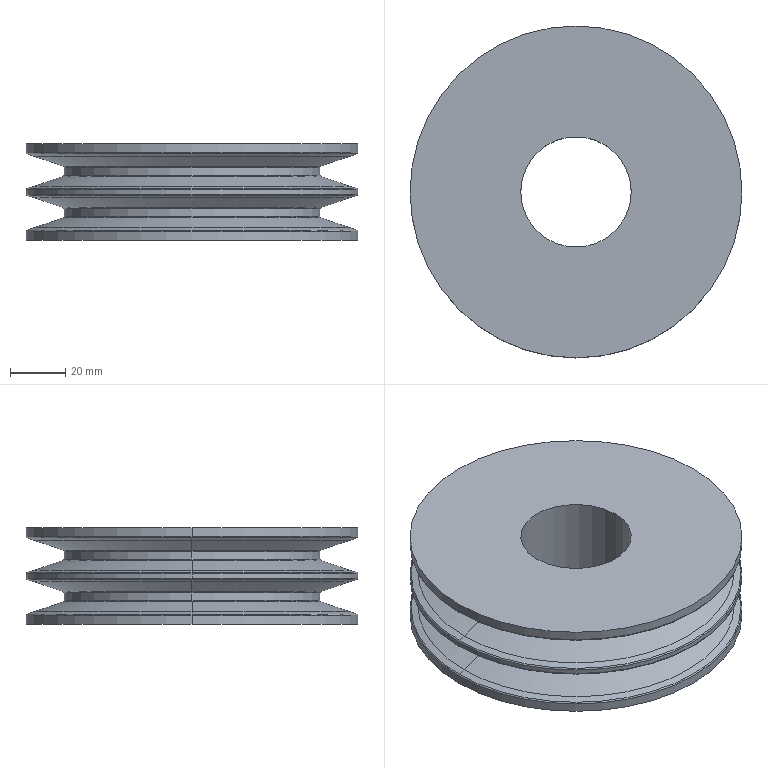Part | SolidWorks | features Extrusion 1, Fillet 1, LPattern 1, RevCut 1 | 1 solid | 46 faces | box 120 x 120 x 35 mm | volume 274896 mm3 | torus 16 | cone 16 | cylinder 12 | plane 2 | commonest cylinder face diameters 120 x6 92.4 x4 40 x2
STEP:
#1=CARTESIAN_POINT('',(-46.537,0.,-5.671));
#2=VERTEX_POINT('',#1);
#3=CARTESIAN_POINT('',(46.537,0.,-5.671));
#4=VERTEX_POINT('',#3);
#5=CARTESIAN_POINT('',(0.,0.,-5.671));
#6=DIRECTION('',(0.,0.,1.));
#7=DIRECTION('',(1.,0.,0.));
#8=AXIS2_PLACEMENT_3D('',#5,#6,#7);
#9=CIRCLE('',#8,46.537);
#10=EDGE_CURVE('',#2,#4,#9,.T.);
#11=ORIENTED_EDGE('',*,*,#10,.F.);
#12=CARTESIAN_POINT('',(-46.2,0.,-6.144));
#13=VERTEX_POINT('',#12);
#14=CARTESIAN_POINT('',(-46.7,0.,-6.144));
#15=DIRECTION('',(0.,1.,0.));
#16=DIRECTION('',(-1.,0.,0.));
#17=AXIS2_PLACEMENT_3D('',#14,#15,#16);
#18=CIRCLE('',#17,0.5);
#19=EDGE_CURVE('',#2,#13,#18,.T.);
#20=ORIENTED_EDGE('',*,*,#19,.T.);
#21=CARTESIAN_POINT('',(46.2,0.,-6.144));
#22=VERTEX_POINT('',#21);
#23=CARTESIAN_POINT('',(0.,0.,-6.144));
#24=DIRECTION('',(0.,0.,-1.));
#25=DIRECTION('',(1.,0.,0.));
#26=AXIS2_PLACEMENT_3D('',#23,#24,#25);
#27=CIRCLE('',#26,46.2);
#28=EDGE_CURVE('',#22,#13,#27,.T.);
#29=ORIENTED_EDGE('',*,*,#28,.F.);
#30=CARTESIAN_POINT('',(46.7,0.,-6.144));
#31=DIRECTION('',(0.,-1.,0.));
#32=DIRECTION('',(0.,0.,-1.));
#33=AXIS2_PLACEMENT_3D('',#30,#31,#32);
#34=CIRCLE('',#33,0.5);
#35=EDGE_CURVE('',#4,#22,#34,.T.);
#36=ORIENTED_EDGE('',*,*,#35,.F.);
#37=EDGE_LOOP('',(#11,#20,#29,#36));
#38=FACE_OUTER_BOUND('',#37,.T.);
#39=CARTESIAN_POINT('',(0.,0.,-6.144));
#40=DIRECTION('',(0.,0.,1.));
#41=DIRECTION('',(1.,0.,0.));
#42=AXIS2_PLACEMENT_3D('',#39,#40,#41);
#43=TOROIDAL_SURFACE('',#42,46.7,0.5);
#44=ADVANCED_FACE('',(#38),#43,.F.);
#45=CARTESIAN_POINT('',(-46.2,0.,-8.856));
#46=VERTEX_POINT('',#45);
#47=CARTESIAN_POINT('',(46.2,0.,-8.856));
#48=VERTEX_POINT('',#47);
#49=CARTESIAN_POINT('',(0.,0.,-8.856));
#50=DIRECTION('',(0.,0.,1.));
#51=DIRECTION('',(1.,0.,0.));
#52=AXIS2_PLACEMENT_3D('',#49,#50,#51);
#53=CIRCLE('',#52,46.2);
#54=EDGE_CURVE('',#46,#48,#53,.T.);
#55=ORIENTED_EDGE('',*,*,#54,.F.);
#56=CARTESIAN_POINT('',(-46.537,0.,-9.329));
#57=VERTEX_POINT('',#56);
#58=CARTESIAN_POINT('',(-46.7,0.,-8.856));
#59=DIRECTION('',(0.,1.,0.));
#60=DIRECTION('',(-1.,0.,0.));
#61=AXIS2_PLACEMENT_3D('',#58,#59,#60);
#62=CIRCLE('',#61,0.5);
#63=EDGE_CURVE('',#46,#57,#62,.T.);
#64=ORIENTED_EDGE('',*,*,#63,.T.);
#65=CARTESIAN_POINT('',(46.537,0.,-9.329));
#66=VERTEX_POINT('',#65);
#67=CARTESIAN_POINT('',(0.,0.,-9.329));
#68=DIRECTION('',(0.,0.,-1.));
#69=DIRECTION('',(-1.,0.,0.));
#70=AXIS2_PLACEMENT_3D('',#67,#68,#69);
#71=CIRCLE('',#70,46.537);
#72=EDGE_CURVE('',#66,#57,#71,.T.);
#73=ORIENTED_EDGE('',*,*,#72,.F.);
#74=CARTESIAN_POINT('',(46.7,0.,-8.856));
#75=DIRECTION('',(0.,-1.,0.));
#76=DIRECTION('',(0.,0.,-1.));
#77=AXIS2_PLACEMENT_3D('',#74,#75,#76);
#78=CIRCLE('',#77,0.5);
#79=EDGE_CURVE('',#48,#66,#78,.T.);
#80=ORIENTED_EDGE('',*,*,#79,.F.);
#81=EDGE_LOOP('',(#55,#64,#73,#80));
#82=FACE_OUTER_BOUND('',#81,.T.);
#83=CARTESIAN_POINT('',(0.,0.,-8.856));
#84=DIRECTION('',(0.,0.,1.));
#85=DIRECTION('',(1.,0.,0.));
#86=AXIS2_PLACEMENT_3D('',#83,#84,#85);
#87=TOROIDAL_SURFACE('',#86,46.7,0.5);
#88=ADVANCED_FACE('',(#82),#87,.F.);
#89=CARTESIAN_POINT('',(60.,0.,-0.7793));
#90=VERTEX_POINT('',#89);
#91=CARTESIAN_POINT('',(-60.,0.,-0.7793));
#92=VERTEX_POINT('',#91);
#93=CARTESIAN_POINT('',(0.,0.,-0.7793));
#94=DIRECTION('',(0.,0.,1.));
#95=DIRECTION('',(-1.,0.,0.));
#96=AXIS2_PLACEMENT_3D('',#93,#94,#95);
#97=CIRCLE('',#96,60.);
#98=EDGE_CURVE('',#90,#92,#97,.T.);
#99=ORIENTED_EDGE('',*,*,#98,.F.);
#100=CARTESIAN_POINT('',(59.645,0.,-1.258));
#101=VERTEX_POINT('',#100);
#102=CARTESIAN_POINT('',(59.5,0.,-0.7793));
#103=DIRECTION('',(0.,1.,0.));
#104=DIRECTION('',(-1.,0.,0.));
#105=AXIS2_PLACEMENT_3D('',#102,#103,#104);
#106=CIRCLE('',#105,0.5);
#107=EDGE_CURVE('',#90,#101,#106,.T.);
#108=ORIENTED_EDGE('',*,*,#107,.T.);
#109=CARTESIAN_POINT('',(-59.645,0.,-1.258));
#110=VERTEX_POINT('',#109);
#111=CARTESIAN_POINT('',(0.,0.,-1.258));
#112=DIRECTION('',(0.,0.,-1.));
#113=DIRECTION('',(1.,0.,0.));
#114=AXIS2_PLACEMENT_3D('',#111,#112,#113);
#115=CIRCLE('',#114,59.645);
#116=EDGE_CURVE('',#110,#101,#115,.T.);
#117=ORIENTED_EDGE('',*,*,#116,.F.);
#118=CARTESIAN_POINT('',(-59.5,0.,-0.7793));
#119=DIRECTION('',(0.,-1.,0.));
#120=DIRECTION('',(0.,0.,-1.));
#121=AXIS2_PLACEMENT_3D('',#118,#119,#120);
#122=CIRCLE('',#121,0.5);
#123=EDGE_CURVE('',#92,#110,#122,.T.);
#124=ORIENTED_EDGE('',*,*,#123,.F.);
#125=EDGE_LOOP('',(#99,#108,#117,#124));
#126=FACE_OUTER_BOUND('',#125,.T.);
#127=CARTESIAN_POINT('',(0.,0.,-0.7793));
#128=DIRECTION('',(0.,0.,-1.));
#129=DIRECTION('',(-1.,0.,0.));
#130=AXIS2_PLACEMENT_3D('',#127,#128,#129);
#131=TOROIDAL_SURFACE('',#130,59.5,0.5);
#132=ADVANCED_FACE('',(#126),#131,.T.);
#133=CARTESIAN_POINT('',(59.645,0.,-13.742));
#134=VERTEX_POINT('',#133);
#135=CARTESIAN_POINT('',(-59.645,0.,-13.742));
#136=VERTEX_POINT('',#135);
#137=CARTESIAN_POINT('',(0.,0.,-13.742));
#138=DIRECTION('',(0.,0.,1.));
#139=DIRECTION('',(-1.,0.,0.));
#140=AXIS2_PLACEMENT_3D('',#137,#138,#139);
#141=CIRCLE('',#140,59.645);
#142=EDGE_CURVE('',#134,#136,#141,.T.);
#143=ORIENTED_EDGE('',*,*,#142,.F.);
#144=CARTESIAN_POINT('',(60.,0.,-14.221));
#145=VERTEX_POINT('',#144);
#146=CARTESIAN_POINT('',(59.5,0.,-14.221));
#147=DIRECTION('',(0.,1.,0.));
#148=DIRECTION('',(-1.,0.,0.));
#149=AXIS2_PLACEMENT_3D('',#146,#147,#148);
#150=CIRCLE('',#149,0.5);
#151=EDGE_CURVE('',#134,#145,#150,.T.);
#152=ORIENTED_EDGE('',*,*,#151,.T.);
#153=CARTESIAN_POINT('',(-60.,0.,-14.221));
#154=VERTEX_POINT('',#153);
#155=CARTESIAN_POINT('',(0.,0.,-14.221));
#156=DIRECTION('',(0.,0.,-1.));
#157=DIRECTION('',(-1.,0.,0.));
#158=AXIS2_PLACEMENT_3D('',#155,#156,#157);
#159=CIRCLE('',#158,60.);
#160=EDGE_CURVE('',#154,#145,#159,.T.);
#161=ORIENTED_EDGE('',*,*,#160,.F.);
#162=CARTESIAN_POINT('',(-59.5,0.,-14.221));
#163=DIRECTION('',(0.,-1.,0.));
#164=DIRECTION('',(0.,0.,-1.));
#165=AXIS2_PLACEMENT_3D('',#162,#163,#164);
#166=CIRCLE('',#165,0.5);
#167=EDGE_CURVE('',#136,#154,#166,.T.);
#168=ORIENTED_EDGE('',*,*,#167,.F.);
#169=EDGE_LOOP('',(#143,#152,#161,#168));
#170=FACE_OUTER_BOUND('',#169,.T.);
#171=CARTESIAN_POINT('',(0.,0.,-14.221));
#172=DIRECTION('',(0.,0.,-1.));
#173=DIRECTION('',(-1.,0.,0.));
#174=AXIS2_PLACEMENT_3D('',#171,#172,#173);
#175=TOROIDAL_SURFACE('',#174,59.5,0.5);
#176=ADVANCED_FACE('',(#170),#175,.T.);
#177=CARTESIAN_POINT('',(57.2,0.,-13.));
#178=VERTEX_POINT('',#177);
#179=CARTESIAN_POINT('',(-57.2,0.,-13.));
#180=VERTEX_POINT('',#179);
#181=CARTESIAN_POINT('',(0.,0.,-13.));
#182=DIRECTION('',(0.,0.,1.));
#183=DIRECTION('',(1.,0.,0.));
#184=AXIS2_PLACEMENT_3D('',#181,#182,#183);
#185=CIRCLE('',#184,57.2);
#186=EDGE_CURVE('',#178,#180,#185,.T.);
#187=ORIENTED_EDGE('',*,*,#186,.F.);
#188=CARTESIAN_POINT('',(57.2,0.,-13.));
#189=DIRECTION('',(0.9569,0.,-0.2905));
#190=VECTOR('',#189,1000.);
#191=LINE('',#188,#190);
#192=EDGE_CURVE('',#178,#134,#191,.T.);
#193=ORIENTED_EDGE('',*,*,#192,.T.);
#194=ORIENTED_EDGE('',*,*,#142,.T.);
#195=CARTESIAN_POINT('',(-57.2,0.,-13.));
#196=DIRECTION('',(-0.9569,0.,-0.2905));
#197=VECTOR('',#196,1000.);
#198=LINE('',#195,#197);
#199=EDGE_CURVE('',#180,#136,#198,.T.);
#200=ORIENTED_EDGE('',*,*,#199,.F.);
#201=EDGE_LOOP('',(#187,#193,#194,#200));
#202=FACE_OUTER_BOUND('',#201,.T.);
#203=CARTESIAN_POINT('',(0.,0.,-13.));
#204=DIRECTION('',(0.,0.,-1.));
#205=DIRECTION('',(-1.,0.,0.));
#206=AXIS2_PLACEMENT_3D('',#203,#204,#205);
#207=CONICAL_SURFACE('',#206,57.2,1.276);
#208=ADVANCED_FACE('',(#202),#207,.T.);
#209=CARTESIAN_POINT('',(0.,0.,-9.329));
#210=DIRECTION('',(0.,0.,-1.));
#211=DIRECTION('',(-1.,0.,0.));
#212=AXIS2_PLACEMENT_3D('',#209,#210,#211);
#213=CIRCLE('',#212,46.537);
#214=EDGE_CURVE('',#57,#66,#213,.T.);
#215=ORIENTED_EDGE('',*,*,#214,.T.);
#216=CARTESIAN_POINT('',(46.2,0.,-9.212));
#217=DIRECTION('',(0.9455,0.,-0.3256));
#218=VECTOR('',#217,1000.);
#219=LINE('',#216,#218);
#220=EDGE_CURVE('',#66,#178,#219,.T.);
#221=ORIENTED_EDGE('',*,*,#220,.T.);
#222=ORIENTED_EDGE('',*,*,#186,.T.);
#223=CARTESIAN_POINT('',(-46.2,0.,-9.212));
#224=DIRECTION('',(-0.9455,0.,-0.3256));
#225=VECTOR('',#224,1000.);
#226=LINE('',#223,#225);
#227=EDGE_CURVE('',#57,#180,#226,.T.);
#228=ORIENTED_EDGE('',*,*,#227,.F.);
#229=EDGE_LOOP('',(#215,#221,#222,#228));
#230=FACE_OUTER_BOUND('',#229,.T.);
#231=CARTESIAN_POINT('',(0.,0.,-9.212));
#232=DIRECTION('',(0.,0.,-1.));
#233=DIRECTION('',(-1.,0.,0.));
#234=AXIS2_PLACEMENT_3D('',#231,#232,#233);
#235=CONICAL_SURFACE('',#234,46.2,1.239);
#236=ADVANCED_FACE('',(#230),#235,.T.);
#237=CARTESIAN_POINT('',(0.,0.,-8.856));
#238=DIRECTION('',(0.,0.,1.));
#239=DIRECTION('',(1.,0.,0.));
#240=AXIS2_PLACEMENT_3D('',#237,#238,#239);
#241=CIRCLE('',#240,46.2);
#242=EDGE_CURVE('',#48,#46,#241,.T.);
#243=ORIENTED_EDGE('',*,*,#242,.T.);
#244=CARTESIAN_POINT('',(-46.2,0.,2.5));
#245=DIRECTION('',(0.,0.,1.));
#246=VECTOR('',#245,1000.);
#247=LINE('',#244,#246);
#248=EDGE_CURVE('',#46,#13,#247,.T.);
#249=ORIENTED_EDGE('',*,*,#248,.T.);
#250=CARTESIAN_POINT('',(0.,0.,-6.144));
#251=DIRECTION('',(0.,0.,-1.));
#252=DIRECTION('',(1.,0.,0.));
#253=AXIS2_PLACEMENT_3D('',#250,#251,#252);
#254=CIRCLE('',#253,46.2);
#255=EDGE_CURVE('',#13,#22,#254,.T.);
#256=ORIENTED_EDGE('',*,*,#255,.T.);
#257=CARTESIAN_POINT('',(46.2,0.,2.5));
#258=DIRECTION('',(0.,0.,1.));
#259=VECTOR('',#258,1000.);
#260=LINE('',#257,#259);
#261=EDGE_CURVE('',#48,#22,#260,.T.);
#262=ORIENTED_EDGE('',*,*,#261,.F.);
#263=EDGE_LOOP('',(#243,#249,#256,#262));
#264=FACE_OUTER_BOUND('',#263,.T.);
#265=CARTESIAN_POINT('',(0.,0.,2.5));
#266=DIRECTION('',(0.,0.,1.));
#267=DIRECTION('',(1.,0.,0.));
#268=AXIS2_PLACEMENT_3D('',#265,#266,#267);
#269=CYLINDRICAL_SURFACE('',#268,46.2);
#270=ADVANCED_FACE('',(#264),#269,.T.);
#271=CARTESIAN_POINT('',(0.,0.,-5.671));
#272=DIRECTION('',(0.,0.,1.));
#273=DIRECTION('',(1.,0.,0.));
#274=AXIS2_PLACEMENT_3D('',#271,#272,#273);
#275=CIRCLE('',#274,46.537);
#276=EDGE_CURVE('',#4,#2,#275,.T.);
#277=ORIENTED_EDGE('',*,*,#276,.T.);
#278=CARTESIAN_POINT('',(-57.2,0.,-2.));
#279=VERTEX_POINT('',#278);
#280=CARTESIAN_POINT('',(-57.2,0.,-2.));
#281=DIRECTION('',(-0.9455,0.,0.3256));
#282=VECTOR('',#281,1000.);
#283=LINE('',#280,#282);
#284=EDGE_CURVE('',#2,#279,#283,.T.);
#285=ORIENTED_EDGE('',*,*,#284,.T.);
#286=CARTESIAN_POINT('',(57.2,0.,-2.));
#287=VERTEX_POINT('',#286);
#288=CARTESIAN_POINT('',(0.,0.,-2.));
#289=DIRECTION('',(0.,0.,1.));
#290=DIRECTION('',(1.,0.,0.));
#291=AXIS2_PLACEMENT_3D('',#288,#289,#290);
#292=CIRCLE('',#291,57.2);
#293=EDGE_CURVE('',#287,#279,#292,.T.);
#294=ORIENTED_EDGE('',*,*,#293,.F.);
#295=CARTESIAN_POINT('',(57.2,0.,-2.));
#296=DIRECTION('',(0.9455,0.,0.3256));
#297=VECTOR('',#296,1000.);
#298=LINE('',#295,#297);
#299=EDGE_CURVE('',#4,#287,#298,.T.);
#300=ORIENTED_EDGE('',*,*,#299,.F.);
#301=EDGE_LOOP('',(#277,#285,#294,#300));
#302=FACE_OUTER_BOUND('',#301,.T.);
#303=CARTESIAN_POINT('',(0.,0.,-2.));
#304=DIRECTION('',(0.,0.,1.));
#305=DIRECTION('',(1.,0.,0.));
#306=AXIS2_PLACEMENT_3D('',#303,#304,#305);
#307=CONICAL_SURFACE('',#306,57.2,1.239);
#308=ADVANCED_FACE('',(#302),#307,.T.);
#309=ORIENTED_EDGE('',*,*,#293,.T.);
#310=CARTESIAN_POINT('',(-60.,0.,-1.15));
#311=DIRECTION('',(-0.9569,0.,0.2905));
#312=VECTOR('',#311,1000.);
#313=LINE('',#310,#312);
#314=EDGE_CURVE('',#279,#110,#313,.T.);
#315=ORIENTED_EDGE('',*,*,#314,.T.);
#316=ORIENTED_EDGE('',*,*,#116,.T.);
#317=CARTESIAN_POINT('',(60.,0.,-1.15));
#318=DIRECTION('',(0.9569,0.,0.2905));
#319=VECTOR('',#318,1000.);
#320=LINE('',#317,#319);
#321=EDGE_CURVE('',#287,#101,#320,.T.);
#322=ORIENTED_EDGE('',*,*,#321,.F.);
#323=EDGE_LOOP('',(#309,#315,#316,#322));
#324=FACE_OUTER_BOUND('',#323,.T.);
#325=CARTESIAN_POINT('',(0.,0.,-1.15));
#326=DIRECTION('',(0.,0.,1.));
#327=DIRECTION('',(1.,0.,0.));
#328=AXIS2_PLACEMENT_3D('',#325,#326,#327);
#329=CONICAL_SURFACE('',#328,60.,1.276);
#330=ADVANCED_FACE('',(#324),#329,.T.);
#331=CARTESIAN_POINT('',(-46.537,0.,9.329));
#332=VERTEX_POINT('',#331);
#333=CARTESIAN_POINT('',(46.537,0.,9.329));
#334=VERTEX_POINT('',#333);
#335=CARTESIAN_POINT('',(0.,0.,9.329));
#336=DIRECTION('',(0.,0.,1.));
#337=DIRECTION('',(1.,0.,0.));
#338=AXIS2_PLACEMENT_3D('',#335,#336,#337);
#339=CIRCLE('',#338,46.537);
#340=EDGE_CURVE('',#332,#334,#339,.T.);
#341=ORIENTED_EDGE('',*,*,#340,.F.);
#342=CARTESIAN_POINT('',(-46.2,0.,8.856));
#343=VERTEX_POINT('',#342);
#344=CARTESIAN_POINT('',(-46.7,0.,8.856));
#345=DIRECTION('',(0.,1.,0.));
#346=DIRECTION('',(-1.,0.,0.));
#347=AXIS2_PLACEMENT_3D('',#344,#345,#346);
#348=CIRCLE('',#347,0.5);
#349=EDGE_CURVE('',#332,#343,#348,.T.);
#350=ORIENTED_EDGE('',*,*,#349,.T.);
#351=CARTESIAN_POINT('',(46.2,0.,8.856));
#352=VERTEX_POINT('',#351);
#353=CARTESIAN_POINT('',(0.,0.,8.856));
#354=DIRECTION('',(0.,0.,-1.));
#355=DIRECTION('',(1.,0.,0.));
#356=AXIS2_PLACEMENT_3D('',#353,#354,#355);
#357=CIRCLE('',#356,46.2);
#358=EDGE_CURVE('',#352,#343,#357,.T.);
#359=ORIENTED_EDGE('',*,*,#358,.F.);
#360=CARTESIAN_POINT('',(46.7,0.,8.856));
#361=DIRECTION('',(0.,-1.,0.));
#362=DIRECTION('',(0.,0.,-1.));
#363=AXIS2_PLACEMENT_3D('',#360,#361,#362);
#364=CIRCLE('',#363,0.5);
#365=EDGE_CURVE('',#334,#352,#364,.T.);
#366=ORIENTED_EDGE('',*,*,#365,.F.);
#367=EDGE_LOOP('',(#341,#350,#359,#366));
#368=FACE_OUTER_BOUND('',#367,.T.);
#369=CARTESIAN_POINT('',(0.,0.,8.856));
#370=DIRECTION('',(0.,0.,1.));
#371=DIRECTION('',(1.,0.,0.));
#372=AXIS2_PLACEMENT_3D('',#369,#370,#371);
#373=TOROIDAL_SURFACE('',#372,46.7,0.5);
#374=ADVANCED_FACE('',(#368),#373,.F.);
#375=CARTESIAN_POINT('',(-46.2,0.,6.144));
#376=VERTEX_POINT('',#375);
#377=CARTESIAN_POINT('',(46.2,0.,6.144));
#378=VERTEX_POINT('',#377);
#379=CARTESIAN_POINT('',(0.,0.,6.144));
#380=DIRECTION('',(0.,0.,1.));
#381=DIRECTION('',(1.,0.,0.));
#382=AXIS2_PLACEMENT_3D('',#379,#380,#381);
#383=CIRCLE('',#382,46.2);
#384=EDGE_CURVE('',#376,#378,#383,.T.);
#385=ORIENTED_EDGE('',*,*,#384,.F.);
#386=CARTESIAN_POINT('',(-46.537,0.,5.671));
#387=VERTEX_POINT('',#386);
#388=CARTESIAN_POINT('',(-46.7,0.,6.144));
#389=DIRECTION('',(0.,1.,0.));
#390=DIRECTION('',(-1.,0.,0.));
#391=AXIS2_PLACEMENT_3D('',#388,#389,#390);
#392=CIRCLE('',#391,0.5);
#393=EDGE_CURVE('',#376,#387,#392,.T.);
#394=ORIENTED_EDGE('',*,*,#393,.T.);
#395=CARTESIAN_POINT('',(46.537,0.,5.671));
#396=VERTEX_POINT('',#395);
#397=CARTESIAN_POINT('',(0.,0.,5.671));
#398=DIRECTION('',(0.,0.,-1.));
#399=DIRECTION('',(-1.,0.,0.));
#400=AXIS2_PLACEMENT_3D('',#397,#398,#399);
#401=CIRCLE('',#400,46.537);
#402=EDGE_CURVE('',#396,#387,#401,.T.);
#403=ORIENTED_EDGE('',*,*,#402,.F.);
#404=CARTESIAN_POINT('',(46.7,0.,6.144));
#405=DIRECTION('',(0.,-1.,0.));
#406=DIRECTION('',(0.,0.,-1.));
#407=AXIS2_PLACEMENT_3D('',#404,#405,#406);
#408=CIRCLE('',#407,0.5);
#409=EDGE_CURVE('',#378,#396,#408,.T.);
#410=ORIENTED_EDGE('',*,*,#409,.F.);
#411=EDGE_LOOP('',(#385,#394,#403,#410));
#412=FACE_OUTER_BOUND('',#411,.T.);
#413=CARTESIAN_POINT('',(0.,0.,6.144));
#414=DIRECTION('',(0.,0.,1.));
#415=DIRECTION('',(1.,0.,0.));
#416=AXIS2_PLACEMENT_3D('',#413,#414,#415);
#417=TOROIDAL_SURFACE('',#416,46.7,0.5);
#418=ADVANCED_FACE('',(#412),#417,.F.);
#419=CARTESIAN_POINT('',(60.,0.,14.221));
#420=VERTEX_POINT('',#419);
#421=CARTESIAN_POINT('',(-60.,0.,14.221));
#422=VERTEX_POINT('',#421);
#423=CARTESIAN_POINT('',(0.,0.,14.221));
#424=DIRECTION('',(0.,0.,1.));
#425=DIRECTION('',(-1.,0.,0.));
#426=AXIS2_PLACEMENT_3D('',#423,#424,#425);
#427=CIRCLE('',#426,60.);
#428=EDGE_CURVE('',#420,#422,#427,.T.);
#429=ORIENTED_EDGE('',*,*,#428,.F.);
#430=CARTESIAN_POINT('',(59.645,0.,13.742));
#431=VERTEX_POINT('',#430);
#432=CARTESIAN_POINT('',(59.5,0.,14.221));
#433=DIRECTION('',(0.,1.,0.));
#434=DIRECTION('',(-1.,0.,0.));
#435=AXIS2_PLACEMENT_3D('',#432,#433,#434);
#436=CIRCLE('',#435,0.5);
#437=EDGE_CURVE('',#420,#431,#436,.T.);
#438=ORIENTED_EDGE('',*,*,#437,.T.);
#439=CARTESIAN_POINT('',(-59.645,0.,13.742));
#440=VERTEX_POINT('',#439);
#441=CARTESIAN_POINT('',(0.,0.,13.742));
#442=DIRECTION('',(0.,0.,-1.));
#443=DIRECTION('',(1.,0.,0.));
#444=AXIS2_PLACEMENT_3D('',#441,#442,#443);
#445=CIRCLE('',#444,59.645);
#446=EDGE_CURVE('',#440,#431,#445,.T.);
#447=ORIENTED_EDGE('',*,*,#446,.F.);
#448=CARTESIAN_POINT('',(-59.5,0.,14.221));
#449=DIRECTION('',(0.,-1.,0.));
#450=DIRECTION('',(0.,0.,-1.));
#451=AXIS2_PLACEMENT_3D('',#448,#449,#450);
#452=CIRCLE('',#451,0.5);
#453=EDGE_CURVE('',#422,#440,#452,.T.);
#454=ORIENTED_EDGE('',*,*,#453,.F.);
#455=EDGE_LOOP('',(#429,#438,#447,#454));
#456=FACE_OUTER_BOUND('',#455,.T.);
#457=CARTESIAN_POINT('',(0.,0.,14.221));
#458=DIRECTION('',(0.,0.,-1.));
#459=DIRECTION('',(-1.,0.,0.));
#460=AXIS2_PLACEMENT_3D('',#457,#458,#459);
#461=TOROIDAL_SURFACE('',#460,59.5,0.5);
#462=ADVANCED_FACE('',(#456),#461,.T.);
#463=CARTESIAN_POINT('',(59.645,0.,1.258));
#464=VERTEX_POINT('',#463);
#465=CARTESIAN_POINT('',(-59.645,0.,1.258));
#466=VERTEX_POINT('',#465);
#467=CARTESIAN_POINT('',(0.,0.,1.258));
#468=DIRECTION('',(0.,0.,1.));
#469=DIRECTION('',(-1.,0.,0.));
#470=AXIS2_PLACEMENT_3D('',#467,#468,#469);
#471=CIRCLE('',#470,59.645);
#472=EDGE_CURVE('',#464,#466,#471,.T.);
#473=ORIENTED_EDGE('',*,*,#472,.F.);
#474=CARTESIAN_POINT('',(60.,0.,0.7793));
#475=VERTEX_POINT('',#474);
#476=CARTESIAN_POINT('',(59.5,0.,0.7793));
#477=DIRECTION('',(0.,1.,0.));
#478=DIRECTION('',(-1.,0.,0.));
#479=AXIS2_PLACEMENT_3D('',#476,#477,#478);
#480=CIRCLE('',#479,0.5);
#481=EDGE_CURVE('',#464,#475,#480,.T.);
#482=ORIENTED_EDGE('',*,*,#481,.T.);
#483=CARTESIAN_POINT('',(-60.,0.,0.7793));
#484=VERTEX_POINT('',#483);
#485=CARTESIAN_POINT('',(0.,0.,0.7793));
#486=DIRECTION('',(0.,0.,-1.));
#487=DIRECTION('',(-1.,0.,0.));
#488=AXIS2_PLACEMENT_3D('',#485,#486,#487);
#489=CIRCLE('',#488,60.);
#490=EDGE_CURVE('',#484,#475,#489,.T.);
#491=ORIENTED_EDGE('',*,*,#490,.F.);
#492=CARTESIAN_POINT('',(-59.5,0.,0.7793));
#493=DIRECTION('',(0.,-1.,0.));
#494=DIRECTION('',(0.,0.,-1.));
#495=AXIS2_PLACEMENT_3D('',#492,#493,#494);
#496=CIRCLE('',#495,0.5);
#497=EDGE_CURVE('',#466,#484,#496,.T.);
#498=ORIENTED_EDGE('',*,*,#497,.F.);
#499=EDGE_LOOP('',(#473,#482,#491,#498));
#500=FACE_OUTER_BOUND('',#499,.T.);
#501=CARTESIAN_POINT('',(0.,0.,0.7793));
#502=DIRECTION('',(0.,0.,-1.));
#503=DIRECTION('',(-1.,0.,0.));
#504=AXIS2_PLACEMENT_3D('',#501,#502,#503);
#505=TOROIDAL_SURFACE('',#504,59.5,0.5);
#506=ADVANCED_FACE('',(#500),#505,.T.);
#507=CARTESIAN_POINT('',(57.2,0.,2.));
#508=VERTEX_POINT('',#507);
#509=CARTESIAN_POINT('',(-57.2,0.,2.));
#510=VERTEX_POINT('',#509);
#511=CARTESIAN_POINT('',(0.,0.,2.));
#512=DIRECTION('',(0.,0.,1.));
#513=DIRECTION('',(1.,0.,0.));
#514=AXIS2_PLACEMENT_3D('',#511,#512,#513);
#515=CIRCLE('',#514,57.2);
#516=EDGE_CURVE('',#508,#510,#515,.T.);
#517=ORIENTED_EDGE('',*,*,#516,.F.);
#518=CARTESIAN_POINT('',(57.2,0.,2.));
#519=DIRECTION('',(0.9569,0.,-0.2905));
#520=VECTOR('',#519,1000.);
#521=LINE('',#518,#520);
#522=EDGE_CURVE('',#508,#464,#521,.T.);
#523=ORIENTED_EDGE('',*,*,#522,.T.);
#524=ORIENTED_EDGE('',*,*,#472,.T.);
#525=CARTESIAN_POINT('',(-57.2,0.,2.));
#526=DIRECTION('',(-0.9569,0.,-0.2905));
#527=VECTOR('',#526,1000.);
#528=LINE('',#525,#527);
#529=EDGE_CURVE('',#510,#466,#528,.T.);
#530=ORIENTED_EDGE('',*,*,#529,.F.);
#531=EDGE_LOOP('',(#517,#523,#524,#530));
#532=FACE_OUTER_BOUND('',#531,.T.);
#533=CARTESIAN_POINT('',(0.,0.,2.));
#534=DIRECTION('',(0.,0.,-1.));
#535=DIRECTION('',(-1.,0.,0.));
#536=AXIS2_PLACEMENT_3D('',#533,#534,#535);
#537=CONICAL_SURFACE('',#536,57.2,1.276);
#538=ADVANCED_FACE('',(#532),#537,.T.);
#539=CARTESIAN_POINT('',(0.,0.,5.671));
#540=DIRECTION('',(0.,0.,-1.));
#541=DIRECTION('',(-1.,0.,0.));
#542=AXIS2_PLACEMENT_3D('',#539,#540,#541);
#543=CIRCLE('',#542,46.537);
#544=EDGE_CURVE('',#387,#396,#543,.T.);
#545=ORIENTED_EDGE('',*,*,#544,.T.);
#546=CARTESIAN_POINT('',(46.2,0.,5.788));
#547=DIRECTION('',(0.9455,0.,-0.3256));
#548=VECTOR('',#547,1000.);
#549=LINE('',#546,#548);
#550=EDGE_CURVE('',#396,#508,#549,.T.);
#551=ORIENTED_EDGE('',*,*,#550,.T.);
#552=ORIENTED_EDGE('',*,*,#516,.T.);
#553=CARTESIAN_POINT('',(-46.2,0.,5.788));
#554=DIRECTION('',(-0.9455,0.,-0.3256));
#555=VECTOR('',#554,1000.);
#556=LINE('',#553,#555);
#557=EDGE_CURVE('',#387,#510,#556,.T.);
#558=ORIENTED_EDGE('',*,*,#557,.F.);
#559=EDGE_LOOP('',(#545,#551,#552,#558));
#560=FACE_OUTER_BOUND('',#559,.T.);
#561=CARTESIAN_POINT('',(0.,0.,5.788));
#562=DIRECTION('',(0.,0.,-1.));
#563=DIRECTION('',(-1.,0.,0.));
#564=AXIS2_PLACEMENT_3D('',#561,#562,#563);
#565=CONICAL_SURFACE('',#564,46.2,1.239);
#566=ADVANCED_FACE('',(#560),#565,.T.);
#567=CARTESIAN_POINT('',(0.,0.,6.144));
#568=DIRECTION('',(0.,0.,1.));
#569=DIRECTION('',(1.,0.,0.));
#570=AXIS2_PLACEMENT_3D('',#567,#568,#569);
#571=CIRCLE('',#570,46.2);
#572=EDGE_CURVE('',#378,#376,#571,.T.);
#573=ORIENTED_EDGE('',*,*,#572,.T.);
#574=CARTESIAN_POINT('',(-46.2,0.,17.5));
#575=DIRECTION('',(0.,0.,1.));
#576=VECTOR('',#575,1000.);
#577=LINE('',#574,#576);
#578=EDGE_CURVE('',#376,#343,#577,.T.);
#579=ORIENTED_EDGE('',*,*,#578,.T.);
#580=CARTESIAN_POINT('',(0.,0.,8.856));
#581=DIRECTION('',(0.,0.,-1.));
#582=DIRECTION('',(1.,0.,0.));
#583=AXIS2_PLACEMENT_3D('',#580,#581,#582);
#584=CIRCLE('',#583,46.2);
#585=EDGE_CURVE('',#343,#352,#584,.T.);
#586=ORIENTED_EDGE('',*,*,#585,.T.);
#587=CARTESIAN_POINT('',(46.2,0.,17.5));
#588=DIRECTION('',(0.,0.,1.));
#589=VECTOR('',#588,1000.);
#590=LINE('',#587,#589);
#591=EDGE_CURVE('',#378,#352,#590,.T.);
#592=ORIENTED_EDGE('',*,*,#591,.F.);
#593=EDGE_LOOP('',(#573,#579,#586,#592));
#594=FACE_OUTER_BOUND('',#593,.T.);
#595=CARTESIAN_POINT('',(0.,0.,17.5));
#596=DIRECTION('',(0.,0.,1.));
#597=DIRECTION('',(1.,0.,0.));
#598=AXIS2_PLACEMENT_3D('',#595,#596,#597);
#599=CYLINDRICAL_SURFACE('',#598,46.2);
#600=ADVANCED_FACE('',(#594),#599,.T.);
#601=CARTESIAN_POINT('',(0.,0.,9.329));
#602=DIRECTION('',(0.,0.,1.));
#603=DIRECTION('',(1.,0.,0.));
#604=AXIS2_PLACEMENT_3D('',#601,#602,#603);
#605=CIRCLE('',#604,46.537);
#606=EDGE_CURVE('',#334,#332,#605,.T.);
#607=ORIENTED_EDGE('',*,*,#606,.T.);
#608=CARTESIAN_POINT('',(-57.2,0.,13.));
#609=VERTEX_POINT('',#608);
#610=CARTESIAN_POINT('',(-57.2,0.,13.));
#611=DIRECTION('',(-0.9455,0.,0.3256));
#612=VECTOR('',#611,1000.);
#613=LINE('',#610,#612);
#614=EDGE_CURVE('',#332,#609,#613,.T.);
#615=ORIENTED_EDGE('',*,*,#614,.T.);
#616=CARTESIAN_POINT('',(57.2,0.,13.));
#617=VERTEX_POINT('',#616);
#618=CARTESIAN_POINT('',(0.,0.,13.));
#619=DIRECTION('',(0.,0.,1.));
#620=DIRECTION('',(1.,0.,0.));
#621=AXIS2_PLACEMENT_3D('',#618,#619,#620);
#622=CIRCLE('',#621,57.2);
#623=EDGE_CURVE('',#617,#609,#622,.T.);
#624=ORIENTED_EDGE('',*,*,#623,.F.);
#625=CARTESIAN_POINT('',(57.2,0.,13.));
#626=DIRECTION('',(0.9455,0.,0.3256));
#627=VECTOR('',#626,1000.);
#628=LINE('',#625,#627);
#629=EDGE_CURVE('',#334,#617,#628,.T.);
#630=ORIENTED_EDGE('',*,*,#629,.F.);
#631=EDGE_LOOP('',(#607,#615,#624,#630));
#632=FACE_OUTER_BOUND('',#631,.T.);
#633=CARTESIAN_POINT('',(0.,0.,13.));
#634=DIRECTION('',(0.,0.,1.));
#635=DIRECTION('',(1.,0.,0.));
#636=AXIS2_PLACEMENT_3D('',#633,#634,#635);
#637=CONICAL_SURFACE('',#636,57.2,1.239);
#638=ADVANCED_FACE('',(#632),#637,.T.);
#639=ORIENTED_EDGE('',*,*,#623,.T.);
#640=CARTESIAN_POINT('',(-60.,0.,13.85));
#641=DIRECTION('',(-0.9569,0.,0.2905));
#642=VECTOR('',#641,1000.);
#643=LINE('',#640,#642);
#644=EDGE_CURVE('',#609,#440,#643,.T.);
#645=ORIENTED_EDGE('',*,*,#644,.T.);
#646=ORIENTED_EDGE('',*,*,#446,.T.);
#647=CARTESIAN_POINT('',(60.,0.,13.85));
#648=DIRECTION('',(0.9569,0.,0.2905));
#649=VECTOR('',#648,1000.);
#650=LINE('',#647,#649);
#651=EDGE_CURVE('',#617,#431,#650,.T.);
#652=ORIENTED_EDGE('',*,*,#651,.F.);
#653=EDGE_LOOP('',(#639,#645,#646,#652));
#654=FACE_OUTER_BOUND('',#653,.T.);
#655=CARTESIAN_POINT('',(0.,0.,13.85));
#656=DIRECTION('',(0.,0.,1.));
#657=DIRECTION('',(1.,0.,0.));
#658=AXIS2_PLACEMENT_3D('',#655,#656,#657);
#659=CONICAL_SURFACE('',#658,60.,1.276);
#660=ADVANCED_FACE('',(#654),#659,.T.);
#661=CARTESIAN_POINT('',(-20.,0.,17.5));
#662=VERTEX_POINT('',#661);
#663=CARTESIAN_POINT('',(20.,0.,17.5));
#664=VERTEX_POINT('',#663);
#665=CARTESIAN_POINT('',(0.,0.,17.5));
#666=DIRECTION('',(0.,0.,1.));
#667=DIRECTION('',(1.,0.,0.));
#668=AXIS2_PLACEMENT_3D('',#665,#666,#667);
#669=CIRCLE('',#668,20.);
#670=EDGE_CURVE('',#662,#664,#669,.T.);
#671=ORIENTED_EDGE('',*,*,#670,.T.);
#672=CARTESIAN_POINT('',(20.,0.,-17.5));
#673=VERTEX_POINT('',#672);
#674=CARTESIAN_POINT('',(20.,0.,17.5));
#675=DIRECTION('',(0.,0.,-1.));
#676=VECTOR('',#675,1000.);
#677=LINE('',#674,#676);
#678=EDGE_CURVE('',#664,#673,#677,.T.);
#679=ORIENTED_EDGE('',*,*,#678,.T.);
#680=CARTESIAN_POINT('',(-20.,0.,-17.5));
#681=VERTEX_POINT('',#680);
#682=CARTESIAN_POINT('',(0.,0.,-17.5));
#683=DIRECTION('',(0.,0.,1.));
#684=DIRECTION('',(1.,0.,0.));
#685=AXIS2_PLACEMENT_3D('',#682,#683,#684);
#686=CIRCLE('',#685,20.);
#687=EDGE_CURVE('',#681,#673,#686,.T.);
#688=ORIENTED_EDGE('',*,*,#687,.F.);
#689=CARTESIAN_POINT('',(-20.,0.,17.5));
#690=DIRECTION('',(0.,0.,-1.));
#691=VECTOR('',#690,1000.);
#692=LINE('',#689,#691);
#693=EDGE_CURVE('',#662,#681,#692,.T.);
#694=ORIENTED_EDGE('',*,*,#693,.F.);
#695=EDGE_LOOP('',(#671,#679,#688,#694));
#696=FACE_OUTER_BOUND('',#695,.T.);
#697=CARTESIAN_POINT('',(0.,0.,17.5));
#698=DIRECTION('',(0.,0.,-1.));
#699=DIRECTION('',(-1.,0.,0.));
#700=AXIS2_PLACEMENT_3D('',#697,#698,#699);
#701=CYLINDRICAL_SURFACE('',#700,20.);
#702=ADVANCED_FACE('',(#696),#701,.F.);
#703=CARTESIAN_POINT('',(60.,0.,17.5));
#704=VERTEX_POINT('',#703);
#705=CARTESIAN_POINT('',(-60.,0.,17.5));
#706=VERTEX_POINT('',#705);
#707=CARTESIAN_POINT('',(0.,0.,17.5));
#708=DIRECTION('',(0.,0.,1.));
#709=DIRECTION('',(1.,0.,0.));
#710=AXIS2_PLACEMENT_3D('',#707,#708,#709);
#711=CIRCLE('',#710,60.);
#712=EDGE_CURVE('',#704,#706,#711,.T.);
#713=ORIENTED_EDGE('',*,*,#712,.F.);
#714=CARTESIAN_POINT('',(60.,0.,17.5));
#715=DIRECTION('',(0.,0.,-1.));
#716=VECTOR('',#715,1000.);
#717=LINE('',#714,#716);
#718=EDGE_CURVE('',#704,#420,#717,.T.);
#719=ORIENTED_EDGE('',*,*,#718,.T.);
#720=ORIENTED_EDGE('',*,*,#428,.T.);
#721=CARTESIAN_POINT('',(-60.,0.,17.5));
#722=DIRECTION('',(0.,0.,-1.));
#723=VECTOR('',#722,1000.);
#724=LINE('',#721,#723);
#725=EDGE_CURVE('',#706,#422,#724,.T.);
#726=ORIENTED_EDGE('',*,*,#725,.F.);
#727=EDGE_LOOP('',(#713,#719,#720,#726));
#728=FACE_OUTER_BOUND('',#727,.T.);
#729=CARTESIAN_POINT('',(0.,0.,17.5));
#730=DIRECTION('',(0.,0.,-1.));
#731=DIRECTION('',(-1.,0.,0.));
#732=AXIS2_PLACEMENT_3D('',#729,#730,#731);
#733=CYLINDRICAL_SURFACE('',#732,60.);
#734=ADVANCED_FACE('',(#728),#733,.T.);
#735=ORIENTED_EDGE('',*,*,#160,.T.);
#736=CARTESIAN_POINT('',(60.,0.,-17.5));
#737=VERTEX_POINT('',#736);
#738=CARTESIAN_POINT('',(60.,0.,17.5));
#739=DIRECTION('',(0.,0.,-1.));
#740=VECTOR('',#739,1000.);
#741=LINE('',#738,#740);
#742=EDGE_CURVE('',#145,#737,#741,.T.);
#743=ORIENTED_EDGE('',*,*,#742,.T.);
#744=CARTESIAN_POINT('',(-60.,0.,-17.5));
#745=VERTEX_POINT('',#744);
#746=CARTESIAN_POINT('',(0.,0.,-17.5));
#747=DIRECTION('',(0.,0.,1.));
#748=DIRECTION('',(1.,0.,0.));
#749=AXIS2_PLACEMENT_3D('',#746,#747,#748);
#750=CIRCLE('',#749,60.);
#751=EDGE_CURVE('',#737,#745,#750,.T.);
#752=ORIENTED_EDGE('',*,*,#751,.T.);
#753=CARTESIAN_POINT('',(-60.,0.,17.5));
#754=DIRECTION('',(0.,0.,-1.));
#755=VECTOR('',#754,1000.);
#756=LINE('',#753,#755);
#757=EDGE_CURVE('',#154,#745,#756,.T.);
#758=ORIENTED_EDGE('',*,*,#757,.F.);
#759=EDGE_LOOP('',(#735,#743,#752,#758));
#760=FACE_OUTER_BOUND('',#759,.T.);
#761=CARTESIAN_POINT('',(0.,0.,17.5));
#762=DIRECTION('',(0.,0.,-1.));
#763=DIRECTION('',(-1.,0.,0.));
#764=AXIS2_PLACEMENT_3D('',#761,#762,#763);
#765=CYLINDRICAL_SURFACE('',#764,60.);
#766=ADVANCED_FACE('',(#760),#765,.T.);
#767=ORIENTED_EDGE('',*,*,#490,.T.);
#768=CARTESIAN_POINT('',(60.,0.,17.5));
#769=DIRECTION('',(0.,0.,-1.));
#770=VECTOR('',#769,1000.);
#771=LINE('',#768,#770);
#772=EDGE_CURVE('',#475,#90,#771,.T.);
#773=ORIENTED_EDGE('',*,*,#772,.T.);
#774=ORIENTED_EDGE('',*,*,#98,.T.);
#775=CARTESIAN_POINT('',(-60.,0.,17.5));
#776=DIRECTION('',(0.,0.,-1.));
#777=VECTOR('',#776,1000.);
#778=LINE('',#775,#777);
#779=EDGE_CURVE('',#484,#92,#778,.T.);
#780=ORIENTED_EDGE('',*,*,#779,.F.);
#781=EDGE_LOOP('',(#767,#773,#774,#780));
#782=FACE_OUTER_BOUND('',#781,.T.);
#783=CARTESIAN_POINT('',(0.,0.,17.5));
#784=DIRECTION('',(0.,0.,-1.));
#785=DIRECTION('',(-1.,0.,0.));
#786=AXIS2_PLACEMENT_3D('',#783,#784,#785);
#787=CYLINDRICAL_SURFACE('',#786,60.);
#788=ADVANCED_FACE('',(#782),#787,.T.);
#789=ORIENTED_EDGE('',*,*,#772,.F.);
#790=CARTESIAN_POINT('',(0.,0.,0.7793));
#791=DIRECTION('',(0.,0.,-1.));
#792=DIRECTION('',(-1.,0.,0.));
#793=AXIS2_PLACEMENT_3D('',#790,#791,#792);
#794=CIRCLE('',#793,60.);
#795=EDGE_CURVE('',#475,#484,#794,.T.);
#796=ORIENTED_EDGE('',*,*,#795,.T.);
#797=ORIENTED_EDGE('',*,*,#779,.T.);
#798=CARTESIAN_POINT('',(0.,0.,-0.7793));
#799=DIRECTION('',(0.,0.,1.));
#800=DIRECTION('',(-1.,0.,0.));
#801=AXIS2_PLACEMENT_3D('',#798,#799,#800);
#802=CIRCLE('',#801,60.);
#803=EDGE_CURVE('',#92,#90,#802,.T.);
#804=ORIENTED_EDGE('',*,*,#803,.T.);
#805=EDGE_LOOP('',(#789,#796,#797,#804));
#806=FACE_OUTER_BOUND('',#805,.T.);
#807=CARTESIAN_POINT('',(0.,0.,17.5));
#808=DIRECTION('',(0.,0.,-1.));
#809=DIRECTION('',(-1.,0.,0.));
#810=AXIS2_PLACEMENT_3D('',#807,#808,#809);
#811=CYLINDRICAL_SURFACE('',#810,60.);
#812=ADVANCED_FACE('',(#806),#811,.T.);
#813=ORIENTED_EDGE('',*,*,#742,.F.);
#814=CARTESIAN_POINT('',(0.,0.,-14.221));
#815=DIRECTION('',(0.,0.,-1.));
#816=DIRECTION('',(-1.,0.,0.));
#817=AXIS2_PLACEMENT_3D('',#814,#815,#816);
#818=CIRCLE('',#817,60.);
#819=EDGE_CURVE('',#145,#154,#818,.T.);
#820=ORIENTED_EDGE('',*,*,#819,.T.);
#821=ORIENTED_EDGE('',*,*,#757,.T.);
#822=CARTESIAN_POINT('',(0.,0.,-17.5));
#823=DIRECTION('',(0.,0.,1.));
#824=DIRECTION('',(1.,0.,0.));
#825=AXIS2_PLACEMENT_3D('',#822,#823,#824);
#826=CIRCLE('',#825,60.);
#827=EDGE_CURVE('',#745,#737,#826,.T.);
#828=ORIENTED_EDGE('',*,*,#827,.T.);
#829=EDGE_LOOP('',(#813,#820,#821,#828));
#830=FACE_OUTER_BOUND('',#829,.T.);
#831=CARTESIAN_POINT('',(0.,0.,17.5));
#832=DIRECTION('',(0.,0.,-1.));
#833=DIRECTION('',(-1.,0.,0.));
#834=AXIS2_PLACEMENT_3D('',#831,#832,#833);
#835=CYLINDRICAL_SURFACE('',#834,60.);
#836=ADVANCED_FACE('',(#830),#835,.T.);
#837=ORIENTED_EDGE('',*,*,#718,.F.);
#838=CARTESIAN_POINT('',(0.,0.,17.5));
#839=DIRECTION('',(0.,0.,1.));
#840=DIRECTION('',(1.,0.,0.));
#841=AXIS2_PLACEMENT_3D('',#838,#839,#840);
#842=CIRCLE('',#841,60.);
#843=EDGE_CURVE('',#706,#704,#842,.T.);
#844=ORIENTED_EDGE('',*,*,#843,.F.);
#845=ORIENTED_EDGE('',*,*,#725,.T.);
#846=CARTESIAN_POINT('',(0.,0.,14.221));
#847=DIRECTION('',(0.,0.,1.));
#848=DIRECTION('',(-1.,0.,0.));
#849=AXIS2_PLACEMENT_3D('',#846,#847,#848);
#850=CIRCLE('',#849,60.);
#851=EDGE_CURVE('',#422,#420,#850,.T.);
#852=ORIENTED_EDGE('',*,*,#851,.T.);
#853=EDGE_LOOP('',(#837,#844,#845,#852));
#854=FACE_OUTER_BOUND('',#853,.T.);
#855=CARTESIAN_POINT('',(0.,0.,17.5));
#856=DIRECTION('',(0.,0.,-1.));
#857=DIRECTION('',(-1.,0.,0.));
#858=AXIS2_PLACEMENT_3D('',#855,#856,#857);
#859=CYLINDRICAL_SURFACE('',#858,60.);
#860=ADVANCED_FACE('',(#854),#859,.T.);
#861=ORIENTED_EDGE('',*,*,#843,.T.);
#862=ORIENTED_EDGE('',*,*,#712,.T.);
#863=EDGE_LOOP('',(#861,#862));
#864=FACE_OUTER_BOUND('',#863,.T.);
#865=ORIENTED_EDGE('',*,*,#670,.F.);
#866=CARTESIAN_POINT('',(0.,0.,17.5));
#867=DIRECTION('',(0.,0.,1.));
#868=DIRECTION('',(1.,0.,0.));
#869=AXIS2_PLACEMENT_3D('',#866,#867,#868);
#870=CIRCLE('',#869,20.);
#871=EDGE_CURVE('',#664,#662,#870,.T.);
#872=ORIENTED_EDGE('',*,*,#871,.F.);
#873=EDGE_LOOP('',(#865,#872));
#874=FACE_BOUND('',#873,.T.);
#875=CARTESIAN_POINT('',(0.,0.,17.5));
#876=DIRECTION('',(0.,0.,1.));
#877=DIRECTION('',(1.,0.,0.));
#878=AXIS2_PLACEMENT_3D('',#875,#876,#877);
#879=PLANE('',#878);
#880=ADVANCED_FACE('',(#864,#874),#879,.T.);
#881=ORIENTED_EDGE('',*,*,#827,.F.);
#882=ORIENTED_EDGE('',*,*,#751,.F.);
#883=EDGE_LOOP('',(#881,#882));
#884=FACE_OUTER_BOUND('',#883,.T.);
#885=ORIENTED_EDGE('',*,*,#687,.T.);
#886=CARTESIAN_POINT('',(0.,0.,-17.5));
#887=DIRECTION('',(0.,0.,1.));
#888=DIRECTION('',(1.,0.,0.));
#889=AXIS2_PLACEMENT_3D('',#886,#887,#888);
#890=CIRCLE('',#889,20.);
#891=EDGE_CURVE('',#673,#681,#890,.T.);
#892=ORIENTED_EDGE('',*,*,#891,.T.);
#893=EDGE_LOOP('',(#885,#892));
#894=FACE_BOUND('',#893,.T.);
#895=CARTESIAN_POINT('',(0.,0.,-17.5));
#896=DIRECTION('',(0.,0.,1.));
#897=DIRECTION('',(1.,0.,0.));
#898=AXIS2_PLACEMENT_3D('',#895,#896,#897);
#899=PLANE('',#898);
#900=ADVANCED_FACE('',(#884,#894),#899,.F.);
#901=ORIENTED_EDGE('',*,*,#678,.F.);
#902=ORIENTED_EDGE('',*,*,#871,.T.);
#903=ORIENTED_EDGE('',*,*,#693,.T.);
#904=ORIENTED_EDGE('',*,*,#891,.F.);
#905=EDGE_LOOP('',(#901,#902,#903,#904));
#906=FACE_OUTER_BOUND('',#905,.T.);
#907=CARTESIAN_POINT('',(0.,0.,17.5));
#908=DIRECTION('',(0.,0.,-1.));
#909=DIRECTION('',(-1.,0.,0.));
#910=AXIS2_PLACEMENT_3D('',#907,#908,#909);
#911=CYLINDRICAL_SURFACE('',#910,20.);
#912=ADVANCED_FACE('',(#906),#911,.F.);
#913=ORIENTED_EDGE('',*,*,#644,.F.);
#914=CARTESIAN_POINT('',(0.,0.,13.));
#915=DIRECTION('',(0.,0.,1.));
#916=DIRECTION('',(1.,0.,0.));
#917=AXIS2_PLACEMENT_3D('',#914,#915,#916);
#918=CIRCLE('',#917,57.2);
#919=EDGE_CURVE('',#609,#617,#918,.T.);
#920=ORIENTED_EDGE('',*,*,#919,.T.);
#921=ORIENTED_EDGE('',*,*,#651,.T.);
#922=CARTESIAN_POINT('',(0.,0.,13.742));
#923=DIRECTION('',(0.,0.,-1.));
#924=DIRECTION('',(1.,0.,0.));
#925=AXIS2_PLACEMENT_3D('',#922,#923,#924);
#926=CIRCLE('',#925,59.645);
#927=EDGE_CURVE('',#431,#440,#926,.T.);
#928=ORIENTED_EDGE('',*,*,#927,.T.);
#929=EDGE_LOOP('',(#913,#920,#921,#928));
#930=FACE_OUTER_BOUND('',#929,.T.);
#931=CARTESIAN_POINT('',(0.,0.,13.85));
#932=DIRECTION('',(0.,0.,1.));
#933=DIRECTION('',(1.,0.,0.));
#934=AXIS2_PLACEMENT_3D('',#931,#932,#933);
#935=CONICAL_SURFACE('',#934,60.,1.276);
#936=ADVANCED_FACE('',(#930),#935,.T.);
#937=ORIENTED_EDGE('',*,*,#614,.F.);
#938=ORIENTED_EDGE('',*,*,#340,.T.);
#939=ORIENTED_EDGE('',*,*,#629,.T.);
#940=ORIENTED_EDGE('',*,*,#919,.F.);
#941=EDGE_LOOP('',(#937,#938,#939,#940));
#942=FACE_OUTER_BOUND('',#941,.T.);
#943=CARTESIAN_POINT('',(0.,0.,13.));
#944=DIRECTION('',(0.,0.,1.));
#945=DIRECTION('',(1.,0.,0.));
#946=AXIS2_PLACEMENT_3D('',#943,#944,#945);
#947=CONICAL_SURFACE('',#946,57.2,1.239);
#948=ADVANCED_FACE('',(#942),#947,.T.);
#949=ORIENTED_EDGE('',*,*,#578,.F.);
#950=ORIENTED_EDGE('',*,*,#384,.T.);
#951=ORIENTED_EDGE('',*,*,#591,.T.);
#952=ORIENTED_EDGE('',*,*,#358,.T.);
#953=EDGE_LOOP('',(#949,#950,#951,#952));
#954=FACE_OUTER_BOUND('',#953,.T.);
#955=CARTESIAN_POINT('',(0.,0.,17.5));
#956=DIRECTION('',(0.,0.,1.));
#957=DIRECTION('',(1.,0.,0.));
#958=AXIS2_PLACEMENT_3D('',#955,#956,#957);
#959=CYLINDRICAL_SURFACE('',#958,46.2);
#960=ADVANCED_FACE('',(#954),#959,.T.);
#961=ORIENTED_EDGE('',*,*,#550,.F.);
#962=ORIENTED_EDGE('',*,*,#402,.T.);
#963=ORIENTED_EDGE('',*,*,#557,.T.);
#964=CARTESIAN_POINT('',(0.,0.,2.));
#965=DIRECTION('',(0.,0.,1.));
#966=DIRECTION('',(1.,0.,0.));
#967=AXIS2_PLACEMENT_3D('',#964,#965,#966);
#968=CIRCLE('',#967,57.2);
#969=EDGE_CURVE('',#510,#508,#968,.T.);
#970=ORIENTED_EDGE('',*,*,#969,.T.);
#971=EDGE_LOOP('',(#961,#962,#963,#970));
#972=FACE_OUTER_BOUND('',#971,.T.);
#973=CARTESIAN_POINT('',(0.,0.,5.788));
#974=DIRECTION('',(0.,0.,-1.));
#975=DIRECTION('',(-1.,0.,0.));
#976=AXIS2_PLACEMENT_3D('',#973,#974,#975);
#977=CONICAL_SURFACE('',#976,46.2,1.239);
#978=ADVANCED_FACE('',(#972),#977,.T.);
#979=ORIENTED_EDGE('',*,*,#522,.F.);
#980=ORIENTED_EDGE('',*,*,#969,.F.);
#981=ORIENTED_EDGE('',*,*,#529,.T.);
#982=CARTESIAN_POINT('',(0.,0.,1.258));
#983=DIRECTION('',(0.,0.,1.));
#984=DIRECTION('',(-1.,0.,0.));
#985=AXIS2_PLACEMENT_3D('',#982,#983,#984);
#986=CIRCLE('',#985,59.645);
#987=EDGE_CURVE('',#466,#464,#986,.T.);
#988=ORIENTED_EDGE('',*,*,#987,.T.);
#989=EDGE_LOOP('',(#979,#980,#981,#988));
#990=FACE_OUTER_BOUND('',#989,.T.);
#991=CARTESIAN_POINT('',(0.,0.,2.));
#992=DIRECTION('',(0.,0.,-1.));
#993=DIRECTION('',(-1.,0.,0.));
#994=AXIS2_PLACEMENT_3D('',#991,#992,#993);
#995=CONICAL_SURFACE('',#994,57.2,1.276);
#996=ADVANCED_FACE('',(#990),#995,.T.);
#997=ORIENTED_EDGE('',*,*,#481,.F.);
#998=ORIENTED_EDGE('',*,*,#987,.F.);
#999=ORIENTED_EDGE('',*,*,#497,.T.);
#1000=ORIENTED_EDGE('',*,*,#795,.F.);
#1001=EDGE_LOOP('',(#997,#998,#999,#1000));
#1002=FACE_OUTER_BOUND('',#1001,.T.);
#1003=CARTESIAN_POINT('',(0.,0.,0.7793));
#1004=DIRECTION('',(0.,0.,-1.));
#1005=DIRECTION('',(-1.,0.,0.));
#1006=AXIS2_PLACEMENT_3D('',#1003,#1004,#1005);
#1007=TOROIDAL_SURFACE('',#1006,59.5,0.5);
#1008=ADVANCED_FACE('',(#1002),#1007,.T.);
#1009=ORIENTED_EDGE('',*,*,#437,.F.);
#1010=ORIENTED_EDGE('',*,*,#851,.F.);
#1011=ORIENTED_EDGE('',*,*,#453,.T.);
#1012=ORIENTED_EDGE('',*,*,#927,.F.);
#1013=EDGE_LOOP('',(#1009,#1010,#1011,#1012));
#1014=FACE_OUTER_BOUND('',#1013,.T.);
#1015=CARTESIAN_POINT('',(0.,0.,14.221));
#1016=DIRECTION('',(0.,0.,-1.));
#1017=DIRECTION('',(-1.,0.,0.));
#1018=AXIS2_PLACEMENT_3D('',#1015,#1016,#1017);
#1019=TOROIDAL_SURFACE('',#1018,59.5,0.5);
#1020=ADVANCED_FACE('',(#1014),#1019,.T.);
#1021=ORIENTED_EDGE('',*,*,#393,.F.);
#1022=ORIENTED_EDGE('',*,*,#572,.F.);
#1023=ORIENTED_EDGE('',*,*,#409,.T.);
#1024=ORIENTED_EDGE('',*,*,#544,.F.);
#1025=EDGE_LOOP('',(#1021,#1022,#1023,#1024));
#1026=FACE_OUTER_BOUND('',#1025,.T.);
#1027=CARTESIAN_POINT('',(0.,0.,6.144));
#1028=DIRECTION('',(0.,0.,1.));
#1029=DIRECTION('',(1.,0.,0.));
#1030=AXIS2_PLACEMENT_3D('',#1027,#1028,#1029);
#1031=TOROIDAL_SURFACE('',#1030,46.7,0.5);
#1032=ADVANCED_FACE('',(#1026),#1031,.F.);
#1033=ORIENTED_EDGE('',*,*,#349,.F.);
#1034=ORIENTED_EDGE('',*,*,#606,.F.);
#1035=ORIENTED_EDGE('',*,*,#365,.T.);
#1036=ORIENTED_EDGE('',*,*,#585,.F.);
#1037=EDGE_LOOP('',(#1033,#1034,#1035,#1036));
#1038=FACE_OUTER_BOUND('',#1037,.T.);
#1039=CARTESIAN_POINT('',(0.,0.,8.856));
#1040=DIRECTION('',(0.,0.,1.));
#1041=DIRECTION('',(1.,0.,0.));
#1042=AXIS2_PLACEMENT_3D('',#1039,#1040,#1041);
#1043=TOROIDAL_SURFACE('',#1042,46.7,0.5);
#1044=ADVANCED_FACE('',(#1038),#1043,.F.);
#1045=ORIENTED_EDGE('',*,*,#314,.F.);
#1046=CARTESIAN_POINT('',(0.,0.,-2.));
#1047=DIRECTION('',(0.,0.,1.));
#1048=DIRECTION('',(1.,0.,0.));
#1049=AXIS2_PLACEMENT_3D('',#1046,#1047,#1048);
#1050=CIRCLE('',#1049,57.2);
#1051=EDGE_CURVE('',#279,#287,#1050,.T.);
#1052=ORIENTED_EDGE('',*,*,#1051,.T.);
#1053=ORIENTED_EDGE('',*,*,#321,.T.);
#1054=CARTESIAN_POINT('',(0.,0.,-1.258));
#1055=DIRECTION('',(0.,0.,-1.));
#1056=DIRECTION('',(1.,0.,0.));
#1057=AXIS2_PLACEMENT_3D('',#1054,#1055,#1056);
#1058=CIRCLE('',#1057,59.645);
#1059=EDGE_CURVE('',#101,#110,#1058,.T.);
#1060=ORIENTED_EDGE('',*,*,#1059,.T.);
#1061=EDGE_LOOP('',(#1045,#1052,#1053,#1060));
#1062=FACE_OUTER_BOUND('',#1061,.T.);
#1063=CARTESIAN_POINT('',(0.,0.,-1.15));
#1064=DIRECTION('',(0.,0.,1.));
#1065=DIRECTION('',(1.,0.,0.));
#1066=AXIS2_PLACEMENT_3D('',#1063,#1064,#1065);
#1067=CONICAL_SURFACE('',#1066,60.,1.276);
#1068=ADVANCED_FACE('',(#1062),#1067,.T.);
#1069=ORIENTED_EDGE('',*,*,#284,.F.);
#1070=ORIENTED_EDGE('',*,*,#10,.T.);
#1071=ORIENTED_EDGE('',*,*,#299,.T.);
#1072=ORIENTED_EDGE('',*,*,#1051,.F.);
#1073=EDGE_LOOP('',(#1069,#1070,#1071,#1072));
#1074=FACE_OUTER_BOUND('',#1073,.T.);
#1075=CARTESIAN_POINT('',(0.,0.,-2.));
#1076=DIRECTION('',(0.,0.,1.));
#1077=DIRECTION('',(1.,0.,0.));
#1078=AXIS2_PLACEMENT_3D('',#1075,#1076,#1077);
#1079=CONICAL_SURFACE('',#1078,57.2,1.239);
#1080=ADVANCED_FACE('',(#1074),#1079,.T.);
#1081=ORIENTED_EDGE('',*,*,#248,.F.);
#1082=ORIENTED_EDGE('',*,*,#54,.T.);
#1083=ORIENTED_EDGE('',*,*,#261,.T.);
#1084=ORIENTED_EDGE('',*,*,#28,.T.);
#1085=EDGE_LOOP('',(#1081,#1082,#1083,#1084));
#1086=FACE_OUTER_BOUND('',#1085,.T.);
#1087=CARTESIAN_POINT('',(0.,0.,2.5));
#1088=DIRECTION('',(0.,0.,1.));
#1089=DIRECTION('',(1.,0.,0.));
#1090=AXIS2_PLACEMENT_3D('',#1087,#1088,#1089);
#1091=CYLINDRICAL_SURFACE('',#1090,46.2);
#1092=ADVANCED_FACE('',(#1086),#1091,.T.);
#1093=ORIENTED_EDGE('',*,*,#220,.F.);
#1094=ORIENTED_EDGE('',*,*,#72,.T.);
#1095=ORIENTED_EDGE('',*,*,#227,.T.);
#1096=CARTESIAN_POINT('',(0.,0.,-13.));
#1097=DIRECTION('',(0.,0.,1.));
#1098=DIRECTION('',(1.,0.,0.));
#1099=AXIS2_PLACEMENT_3D('',#1096,#1097,#1098);
#1100=CIRCLE('',#1099,57.2);
#1101=EDGE_CURVE('',#180,#178,#1100,.T.);
#1102=ORIENTED_EDGE('',*,*,#1101,.T.);
#1103=EDGE_LOOP('',(#1093,#1094,#1095,#1102));
#1104=FACE_OUTER_BOUND('',#1103,.T.);
#1105=CARTESIAN_POINT('',(0.,0.,-9.212));
#1106=DIRECTION('',(0.,0.,-1.));
#1107=DIRECTION('',(-1.,0.,0.));
#1108=AXIS2_PLACEMENT_3D('',#1105,#1106,#1107);
#1109=CONICAL_SURFACE('',#1108,46.2,1.239);
#1110=ADVANCED_FACE('',(#1104),#1109,.T.);
#1111=ORIENTED_EDGE('',*,*,#192,.F.);
#1112=ORIENTED_EDGE('',*,*,#1101,.F.);
#1113=ORIENTED_EDGE('',*,*,#199,.T.);
#1114=CARTESIAN_POINT('',(0.,0.,-13.742));
#1115=DIRECTION('',(0.,0.,1.));
#1116=DIRECTION('',(-1.,0.,0.));
#1117=AXIS2_PLACEMENT_3D('',#1114,#1115,#1116);
#1118=CIRCLE('',#1117,59.645);
#1119=EDGE_CURVE('',#136,#134,#1118,.T.);
#1120=ORIENTED_EDGE('',*,*,#1119,.T.);
#1121=EDGE_LOOP('',(#1111,#1112,#1113,#1120));
#1122=FACE_OUTER_BOUND('',#1121,.T.);
#1123=CARTESIAN_POINT('',(0.,0.,-13.));
#1124=DIRECTION('',(0.,0.,-1.));
#1125=DIRECTION('',(-1.,0.,0.));
#1126=AXIS2_PLACEMENT_3D('',#1123,#1124,#1125);
#1127=CONICAL_SURFACE('',#1126,57.2,1.276);
#1128=ADVANCED_FACE('',(#1122),#1127,.T.);
#1129=ORIENTED_EDGE('',*,*,#151,.F.);
#1130=ORIENTED_EDGE('',*,*,#1119,.F.);
#1131=ORIENTED_EDGE('',*,*,#167,.T.);
#1132=ORIENTED_EDGE('',*,*,#819,.F.);
#1133=EDGE_LOOP('',(#1129,#1130,#1131,#1132));
#1134=FACE_OUTER_BOUND('',#1133,.T.);
#1135=CARTESIAN_POINT('',(0.,0.,-14.221));
#1136=DIRECTION('',(0.,0.,-1.));
#1137=DIRECTION('',(-1.,0.,0.));
#1138=AXIS2_PLACEMENT_3D('',#1135,#1136,#1137);
#1139=TOROIDAL_SURFACE('',#1138,59.5,0.5);
#1140=ADVANCED_FACE('',(#1134),#1139,.T.);
#1141=ORIENTED_EDGE('',*,*,#107,.F.);
#1142=ORIENTED_EDGE('',*,*,#803,.F.);
#1143=ORIENTED_EDGE('',*,*,#123,.T.);
#1144=ORIENTED_EDGE('',*,*,#1059,.F.);
#1145=EDGE_LOOP('',(#1141,#1142,#1143,#1144));
#1146=FACE_OUTER_BOUND('',#1145,.T.);
#1147=CARTESIAN_POINT('',(0.,0.,-0.7793));
#1148=DIRECTION('',(0.,0.,-1.));
#1149=DIRECTION('',(-1.,0.,0.));
#1150=AXIS2_PLACEMENT_3D('',#1147,#1148,#1149);
#1151=TOROIDAL_SURFACE('',#1150,59.5,0.5);
#1152=ADVANCED_FACE('',(#1146),#1151,.T.);
#1153=ORIENTED_EDGE('',*,*,#63,.F.);
#1154=ORIENTED_EDGE('',*,*,#242,.F.);
#1155=ORIENTED_EDGE('',*,*,#79,.T.);
#1156=ORIENTED_EDGE('',*,*,#214,.F.);
#1157=EDGE_LOOP('',(#1153,#1154,#1155,#1156));
#1158=FACE_OUTER_BOUND('',#1157,.T.);
#1159=CARTESIAN_POINT('',(0.,0.,-8.856));
#1160=DIRECTION('',(0.,0.,1.));
#1161=DIRECTION('',(1.,0.,0.));
#1162=AXIS2_PLACEMENT_3D('',#1159,#1160,#1161);
#1163=TOROIDAL_SURFACE('',#1162,46.7,0.5);
#1164=ADVANCED_FACE('',(#1158),#1163,.F.);
#1165=ORIENTED_EDGE('',*,*,#19,.F.);
#1166=ORIENTED_EDGE('',*,*,#276,.F.);
#1167=ORIENTED_EDGE('',*,*,#35,.T.);
#1168=ORIENTED_EDGE('',*,*,#255,.F.);
#1169=EDGE_LOOP('',(#1165,#1166,#1167,#1168));
#1170=FACE_OUTER_BOUND('',#1169,.T.);
#1171=CARTESIAN_POINT('',(0.,0.,-6.144));
#1172=DIRECTION('',(0.,0.,1.));
#1173=DIRECTION('',(1.,0.,0.));
#1174=AXIS2_PLACEMENT_3D('',#1171,#1172,#1173);
#1175=TOROIDAL_SURFACE('',#1174,46.7,0.5);
#1176=ADVANCED_FACE('',(#1170),#1175,.F.);
#1177=CLOSED_SHELL('',(#44,#88,#132,#176,#208,#236,#270,#308,#330,#374,#418,#462,#506,#538,#566,#600,#638,#660,#702,#734,#766,#788,#812,#836,#860,#880,#900,#912,#936,#948,#960,#978,#996,#1008,#1020,#1032,#1044,#1068,#1080,#1092,#1110,#1128,#1140,#1152,#1164,#1176));
#1178=MANIFOLD_SOLID_BREP('',#1177);
#1179=CARTESIAN_POINT('',(0.,0.,0.));
#1180=DIRECTION('',(0.,0.,1.));
#1181=DIRECTION('',(1.,0.,0.));
#1182=AXIS2_PLACEMENT_3D('',#1179,#1180,#1181);
#1183=(LENGTH_UNIT()NAMED_UNIT(*)SI_UNIT(.MILLI.,.METRE.));
#1184=UNCERTAINTY_MEASURE_WITH_UNIT(LENGTH_MEASURE(0.00001),#1183,'','');
#1185=(NAMED_UNIT(*)PLANE_ANGLE_UNIT()SI_UNIT($,.RADIAN.));
#1186=(NAMED_UNIT(*)SI_UNIT($,.STERADIAN.)SOLID_ANGLE_UNIT());
#1187=(GEOMETRIC_REPRESENTATION_CONTEXT(3)GLOBAL_UNCERTAINTY_ASSIGNED_CONTEXT((#1184))GLOBAL_UNIT_ASSIGNED_CONTEXT((#1183,#1185,#1186))REPRESENTATION_CONTEXT('',''));
#1188=ADVANCED_BREP_SHAPE_REPRESENTATION('',(#1178,#1182),#1187);